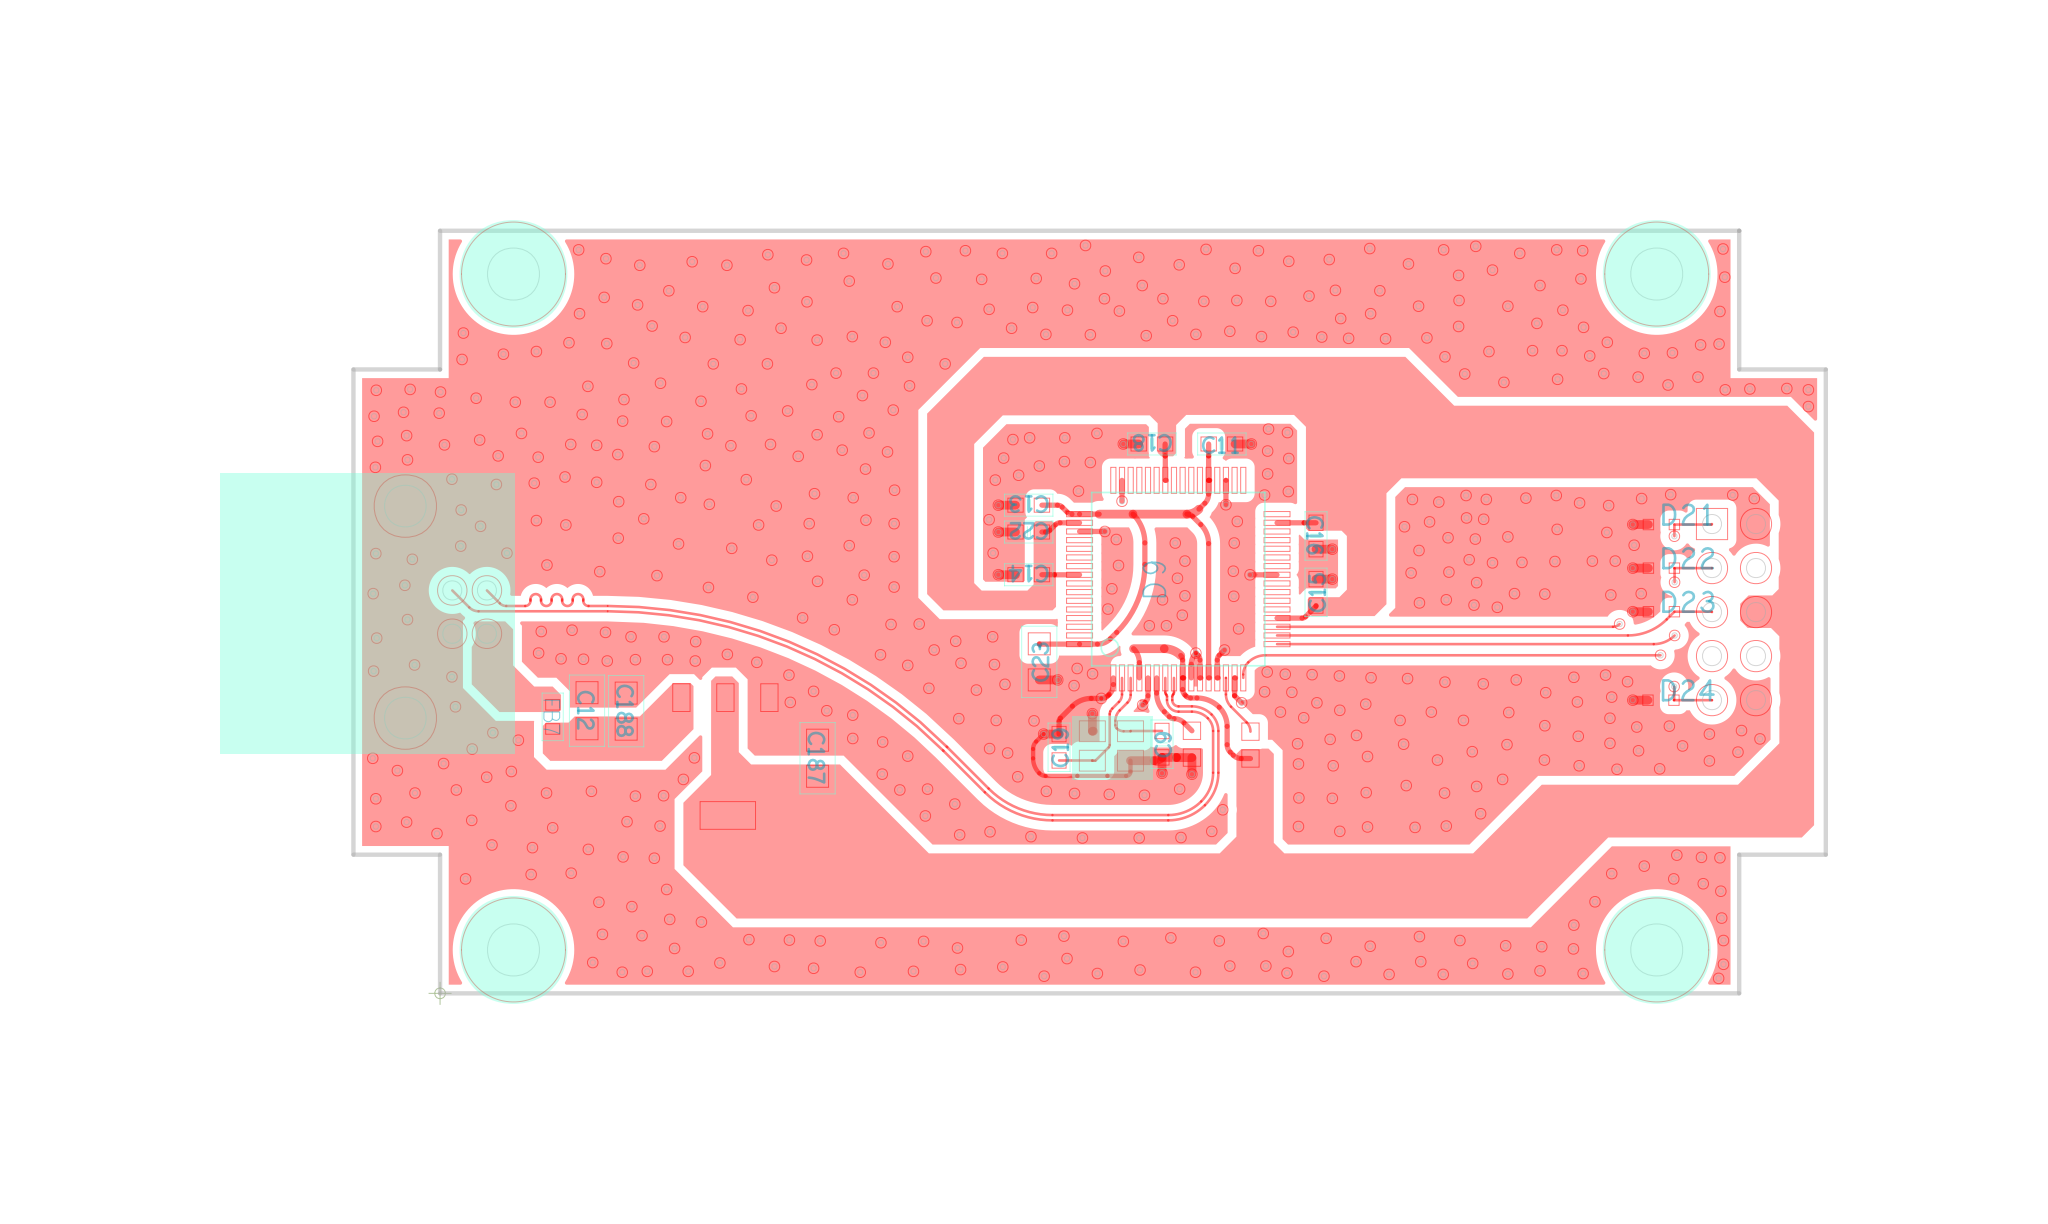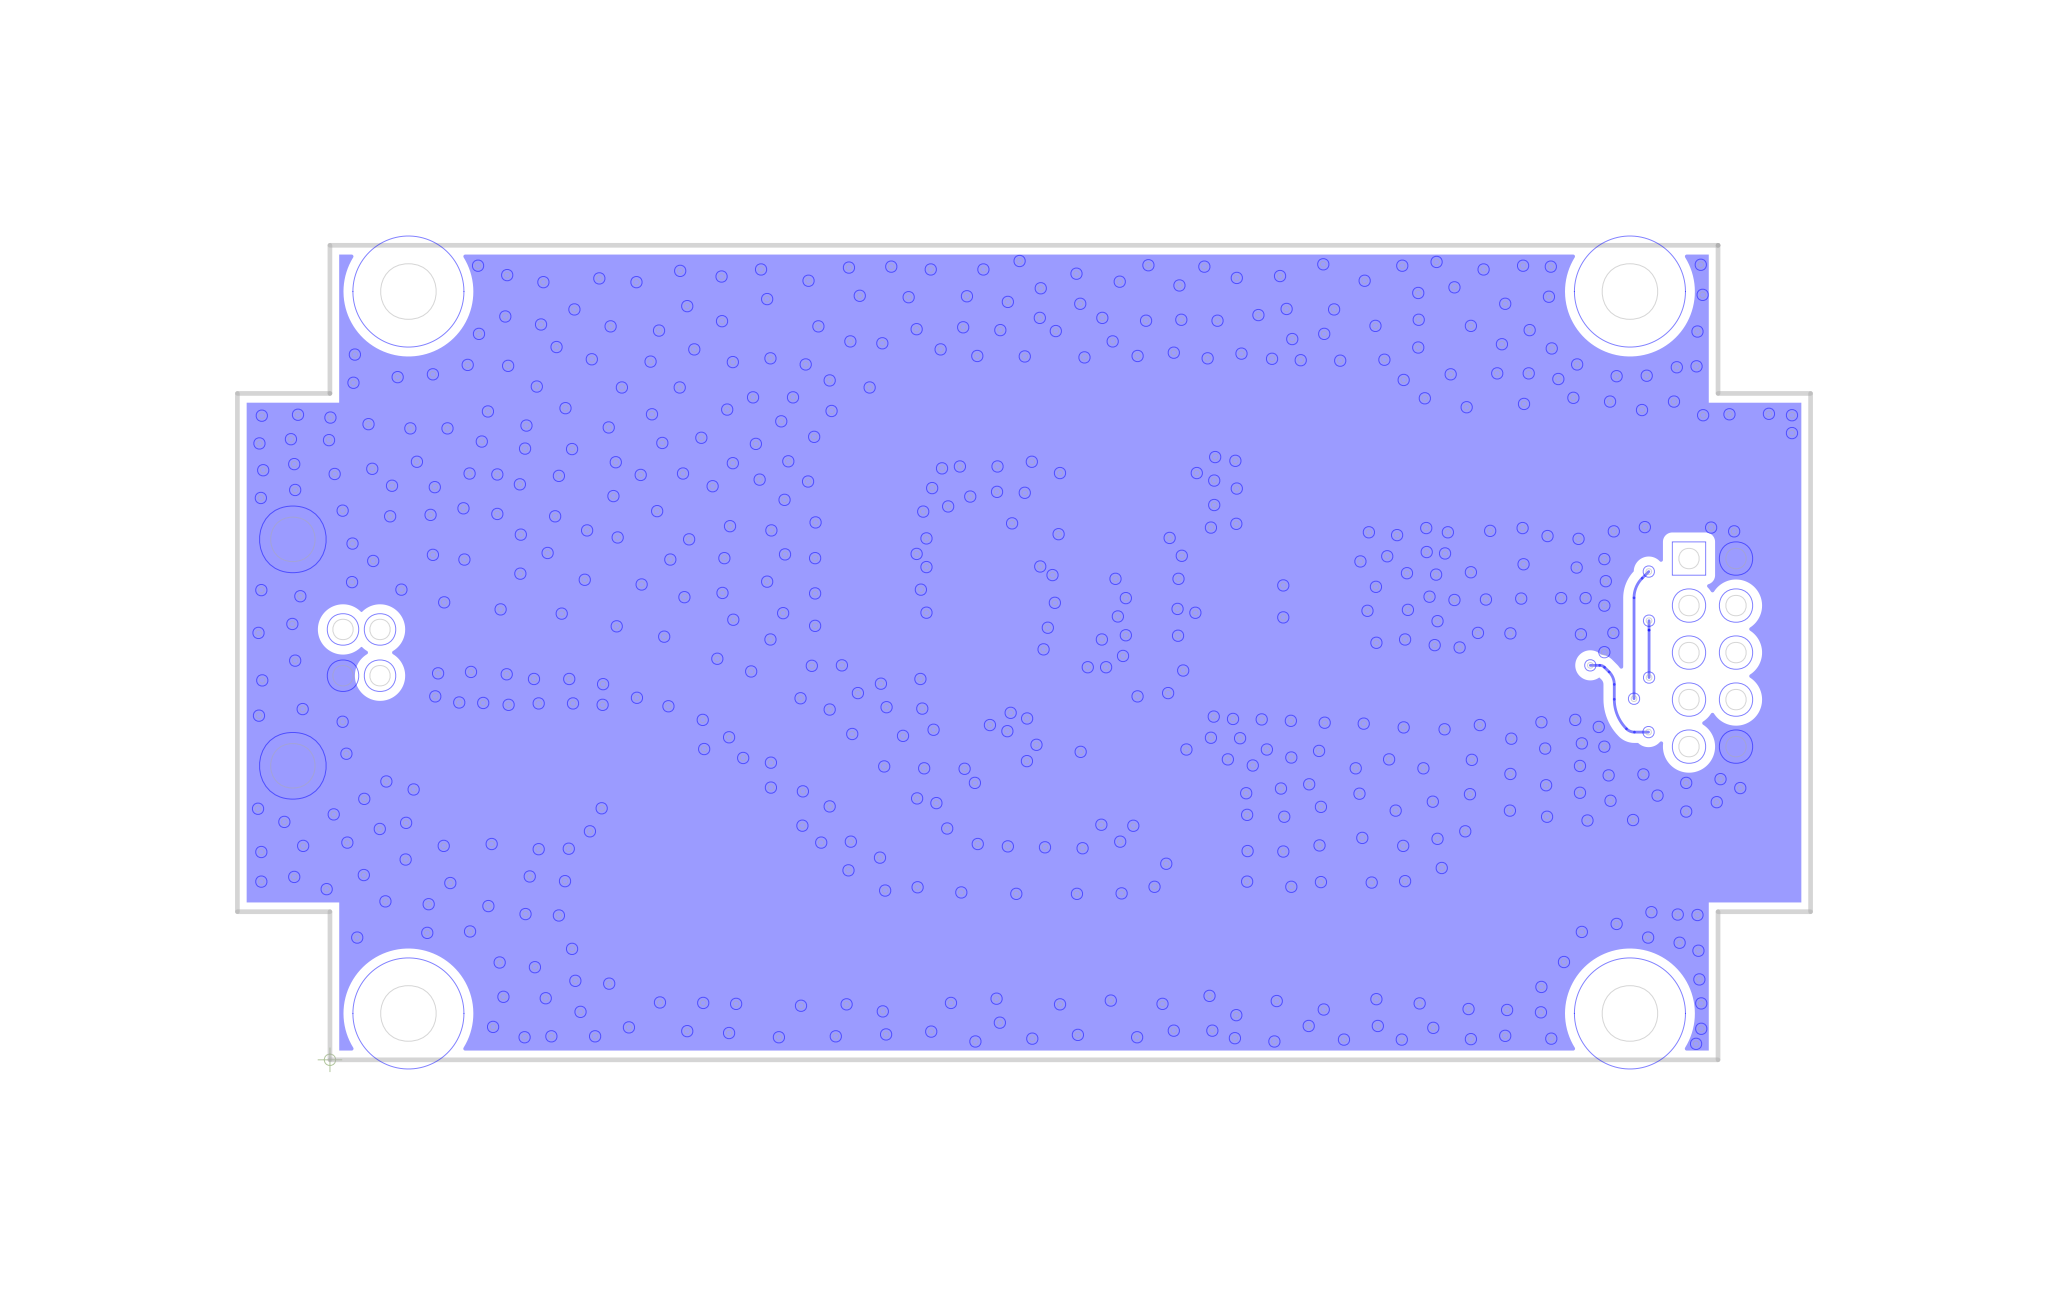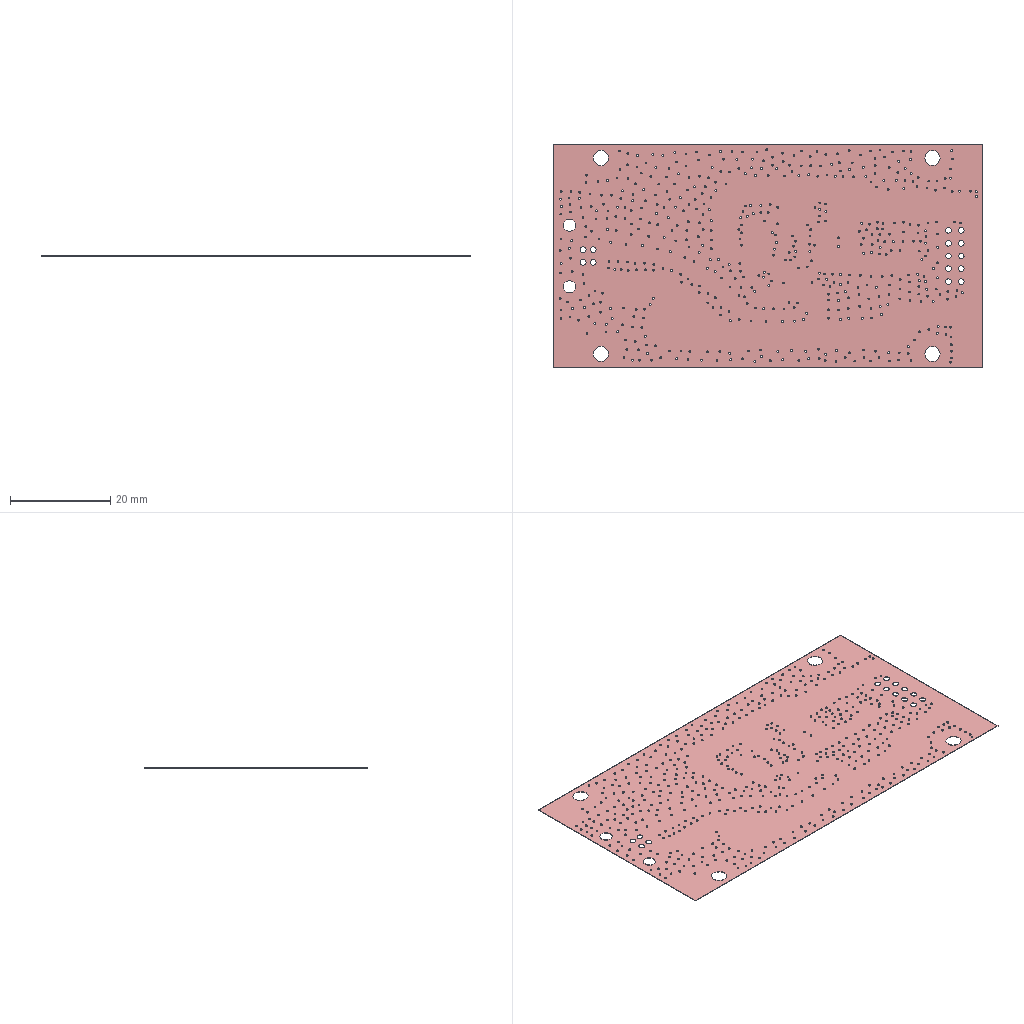Circuit board layout | Cadence Allegro | box 85.3 x 44.3 x 0.1 mm
Layer stack:
# Cadence Allegro layer stack of  (unit mm; from the constraint file cross-section; dielectric type: 0 not recorded (Allegro does not mark core vs prepreg), 3 surface material)
index,name,kind,layer,copper_thickness_mm,dielectric_type,dielectric_thickness_mm,dielectric_material,dielectric_constant
0,Top Surface,other,,,,,,
1,TOP,copper,TOP,0.035,,,,
2,Dielectric1,dielectric,,,0,0.1,FR-4,4.5
3,BOTTOM,copper,BOTTOM,0.035,,,,
4,Bottom Surface,other,,,,,,
# drill layer pairs: low layer,high layer
drill_pair,TOP,BOTTOM
Part placement:
REFDES,COMP_VALUE,SYM_NAME,SYM_X,SYM_Y,SYM_ROTATE,SYM_MIRROR
C9,22pF,SMC0603,1640.902,566.000,90.000,NO
C11,10nF,SMC0603,1776.902,1248.000,0.000,NO
C12,10uF,C0805,334.000,642.098,270.000,NO
C13,100nF,SMC0603,1337.902,1109.000,180.000,NO
C14,100nF,SMC0603,1337.902,951.000,180.000,NO
C15,100nF,SMC0603,1990.902,911.000,90.000,NO
C16,100nF,SMC0603,1990.902,1039.000,270.000,NO
C18,100nF,SMC0603,1617.902,1248.000,180.000,NO
C19,22pF,SMC0603,1406.902,559.000,90.000,NO
C22,100nF,SMC0603,1337.902,1048.000,180.000,NO
C23,10uF,C0805,1361.902,753.000,90.000,NO
C187,10uF,C0805,858.000,534.098,270.000,NO
C188,10uF,C0805,423.000,641.098,270.000,NO
D9,FT2232HL,LQFP64_D12_E12_P0R5,1677.902,941.000,90.000,NO
D20,AMS1117-3.3,SOT-223,654.000,404.098,180.000,NO
D21,BSD5C031V,SOD-523_L1_2-W0_8-LS1_6-BI,2775.902,1065.000,0.000,NO
D22,BSD5C031V,SOD-523_L1_2-W0_8-LS1_6-BI,2775.902,966.000,0.000,NO
D23,BSD5C031V,SOD-523_L1_2-W0_8-LS1_6-BI,2775.902,867.000,0.000,NO
D24,BSD5C031V,SOD-523_L1_2-W0_8-LS1_6-BI,2774.902,666.000,0.000,NO
FB7,MPZ1608S601A NC,FB0603,256.000,628.098,270.000,NO
G1,X322525MSB4SI_C13740,3225,1525.902,562.000,0.000,NO
J1,2.54mm_2x5,IDC-TH_10P-P2_54-H-R2-C5-S2_54,2940.945,866.142,90.000,NO
R185,12K,R0603,1708.902,566.000,90.000,NO
R197,10K,R0603,1841.902,564.000,90.000,NO
X15,usb2.0_B_C46392,USB-B_TH_BF90,13.780,866.142,270.000,NO
Pad and via stacks:
# Allegro (Cadence) via spans and padstacks; design units: ("mils" 3 1000)
# via spans: padstack,start_layer,end_layer,net_example,count
VIA12_24,ETCH/TOP,ETCH/BOTTOM,GND,568
# Allegro padstack definitions: name,start_layer,end_layer,drill,plating,holeType,type
SMD_OV36X30,"ETCH/TOP","ETCH/TOP",0.0,"PLATED","none","smd"
SMD_SQ50,"ETCH/TOP","ETCH/TOP",0.0,"PLATED","none","smd"
SMD10X16,"ETCH/TOP","ETCH/TOP",0.0,"PLATED","none","smd"
SMD32X16,"ETCH/TOP","ETCH/TOP",0.0,"PLATED","none","smd"
SMD0_3X1_5,"ETCH/TOP","ETCH/TOP",0.0,"PLATED","none","smd"
R150_30,"ETCH/TOP","ETCH/TOP",0.0,"PLATED","none","smd"
RECT24X32,"ETCH/TOP","ETCH/TOP",0.0,"PLATED","none","smd"
RECT71X47,"ETCH/TOP","ETCH/TOP",0.0,"PLATED","none","smd"
SMD66X71,"ETCH/TOP","ETCH/TOP",0.0,"PLATED","none","smd"
SMD_SQ32,"ETCH/TOP","ETCH/TOP",0.0,"PLATED","none","smd"
SMD39SQU,"ETCH/TOP","ETCH/TOP",0.0,"NON_PLATED","none","smd"
RECT83X55,"ETCH/TOP","ETCH/TOP",0.0,"PLATED","none","smd"
RE98_42X78_74,"ETCH/TOP","ETCH/TOP",0.0,"NON_PLATED","none","smd"
RE118_11X19_68,"ETCH/TOP","ETCH/TOP",0.0,"NON_PLATED","none","smd"
RECT35X32,"ETCH/TOP","ETCH/TOP",0.0,"PLATED","none","smd"
R150X121,"ETCH/TOP","ETCH/TOP",0.0,"PLATED","none","smd"
SMD_S236P0S40,"ETCH/TOP","ETCH/TOP",0.0,"PLATED","none","smd"
PAD1_8CIR1,"ETCH/TOP","ETCH/BOTTOM",39.402,"PLATED","circle_drill","through"
C054_039,"ETCH/TOP","ETCH/BOTTOM",39.0,"PLATED","circle_drill","through"
S054_039,"ETCH/TOP","ETCH/BOTTOM",39.0,"PLATED","circle_drill","through"
S058_043,"ETCH/TOP","ETCH/BOTTOM",43.0,"PLATED","circle_drill","through"
C058_043,"ETCH/TOP","ETCH/BOTTOM",43.0,"PLATED","circle_drill","through"
VIA,"ETCH/TOP","ETCH/BOTTOM",13.0,"PLATED","circle_drill","through"
TH3P0,"ETCH/TOP","ETCH/BOTTOM",118.11,"PLATED","circle_drill","through"
PLACE-LED3UNIT,"ETCH/TOP","ETCH/BOTTOM",137.799,"PLATED","circle_drill","through"
TH138_CIR118,"ETCH/TOP","ETCH/BOTTOM",137.799,"PLATED","circle_drill","through"
HOLE3P0,"ETCH/TOP","ETCH/BOTTOM",118.11,"PLATED","circle_drill","through"
VIA_10_18,"ETCH/TOP","ETCH/BOTTOM",10.0,"PLATED","circle_drill","through"
PAD60CIR40D_1,"ETCH/TOP","ETCH/BOTTOM",40.0,"PLATED","circle_drill","through"
PAD60SQ40D_1,"ETCH/TOP","ETCH/BOTTOM",40.0,"PLATED","circle_drill","through"
PTH_C669SLOT433X433S40,"ETCH/TOP","ETCH/BOTTOM",43.311,"PLATED","oval slot","through"
PTH_C1221SLOT827X827S40,"ETCH/TOP","ETCH/BOTTOM",82.681,"PLATED","oval slot","through"
HOLE2-3_5,"ETCH/TOP","ETCH/BOTTOM",82.681,"PLATED","circle_drill","through"
PAD158CIR107D,"ETCH/TOP","ETCH/BOTTOM",106.299,"PLATED","circle_drill","through"
VIA12_24,"ETCH/TOP","ETCH/BOTTOM",12.0,"PLATED","circle_drill","through"
PTH_C1417SLOT945X945S40,"ETCH/TOP","ETCH/BOTTOM",94.488,"PLATED","oval slot","through"
PTH_C709SLOT433X433S40,"ETCH/TOP","ETCH/BOTTOM",43.311,"PLATED","oval slot","through"
PTH_S709SLOT433X433S40,"ETCH/TOP","ETCH/BOTTOM",43.311,"PLATED","oval slot","through"
D3,"ETCH/TOP","ETCH/BOTTOM",118.11,"NON_PLATED","circle_drill","through"
C177_17D137_80,"ETCH/TOP","ETCH/BOTTOM",157.48,"PLATED","circle_drill","through"
HOLE5P5D3P2,"ETCH/TOP","ETCH/BOTTOM",125.98,"PLATED","circle_drill","through"
Y300_600,"ETCH/TOP","ETCH/BOTTOM",118.11,"PLATED","circle_drill","through"
Design rules, without the lines most boards share, first 13 of 24 lines:
# Cadence Allegro design rules of  (from the Constraint Manager export constraints.dcfx, design unit mil; typed fields in mm)
# columns: name | kind | enabled | priority | scope1 | scope2 | descriptor | typed fields (field=value)
# Allegro precedence (priority 1 wins): 1 Region class-to-class, 2 Region class, 3 Region, 4 class-to-class, 5 DiffPair/Bus/NetGroup override, 6 NetClass, 7 constraint set (CSet) default
# per-layer values are written LAYER=value in the descriptor and LAYER:mm in the typed field; a maximum of 0 means no limit set
# --- net classes (and buses / net groups) ---
# (no net classes defined: every net uses the default constraint sets)
# --- track widths, neck and differential-pair gap (physical constraint sets) ---
DEFAULT | PhysicalCSet | enabled | 7 | Design default | All | Physical Constraint (Min Line Width=6mil) (Max Line Width=0mil) (Min Neck Width=6mil) (Max Neck Length=0mil) (DiffPair Primary Gap=6mil) (DiffPair Neck Gap=0mil) (DiffPair Min Space=0mil) (DiffPair Coupled +Tol=0mil) (DiffPair Coupled -Tol=0mil) (Min BB Via Stagger=5mil) (Max BB Via Stagger=0mil) (T-junctions=ANYWHERE) (Pad-pad direct connect=ALL_ALLOWED) (Allowed vias=VIA12_24) | min_line_width=0.1524 min_neck_width=0.1524 ts_allowed=ANYWHERE min_bvia_stagger=0.127 max_bvia_stagger=0 diffp_primary_gap=0.1524 diffp_neck_gap=0 diffp_coupled_plus=0 diffp_coupled_minus=0 diffp_min_space=0 max_line_width=0 maximum_neck_length=0 allow_on_etch_subclass=TRUE pad_pad_direct_connect=ALL_ALLOWED vias=VIA12_24
# --- clearances: line / pad / via / shape / hole (spacing constraint sets) ---
DEFAULT | SpacingCSet | enabled | 7 | Design default | All | Clearance Constraint (Line-Line=6mil) (Line-SMD Pad=6mil) (Line-Thru Pin=6mil) (Line-Via=6mil) (Line-Shape=20mil) (SMD Pad-SMD Pad=6mil) (Thru Pin-Thru Pin=6mil) (Thru Pin-SMD Pad=6mil) (SMD Pad-Via=6mil) (Thru Pin-Via=6mil) (Via-Via=6mil) (Shape-SMD Pad=20mil) (Shape-Thru Pin=20mil) (Shape-Via=20mil) (Shape-Shape=20mil) (Hole-Hole=8mil) (Hole-Line=6mil) (Hole-Shape=8mil) (BB Via-BB Via=6mil) (uVia-uVia=5mil) | line_to_line_spacing=0.1524 line_to_smdpin_spacing=0.1524 smdpin_to_smdpin_spacing=0.1524 line_to_testpin_spacing=0.1524 testpin_to_thrupin_spacing=0.1524 testpin_to_testpin_spacing=0.1524 line_to_thruvia_spacing=0.1524 smdpin_to_thruvia_spacing=0.1524 testpin_to_thruvia_spacing=0.1524 thruvia_to_thruvia_spacing=0.1524 bbv_to_line_spacing=0.1524 bbv_to_thrupin_spacing=0.1524 bbv_to_smdpin_spacing=0.1524 bbv_to_testpin_spacing=0.1524 bbv_to_bbv_spacing=0.1524 line_to_testvia_spacing=0.1524 smdpin_to_testvia_spacing=0.1524 testpin_to_testvia_spacing=0.1524 testvia_to_thruvia_spacing=0.1524 bbv_to_testvia_spacing=0.1524 testvia_to_testvia_spacing=0.1524 mvia_to_line_spacing=0.1524 mvia_to_thrupin_spacing=0.127 mvia_to_smdpin_spacing=0.127 mvia_to_testpin_spacing=0.127 mvia_to_thruvia_spacing=0.127 mvia_to_bbv_spacing=0.127 mvia_to_mvia_spacing=0.127 line_to_shape_spacing=0.508 shape_to_smdpin_spacing=0.508 shape_to_testpin_spacing=0.508 shape_to_thruvia_spacing=0.508 bbv_to_shape_spacing=0.508 shape_to_testvia_spacing=0.508 mvia_to_shape_spacing=0.127 shape_to_shape_spacing=0.508 bondpad_to_line_spacing=0.1524 thrupin_to_bondpad_spacing=0.1524 smdpin_to_bondpad_spacing=0.1524 bondpad_to_testpin_spacing=0.1524 bondpad_to_thruvia_spacing=0.1524 bondpad_to_bbv_spacing=0.1524 bondpad_to_testvia_spacing=0.1524 bondpad_to_mvia_spacing=0.127 bondpad_to_bondpad_spacing=0.1524 thrupin_to_thrupin_spacing=0.1524 thrupin_to_smdpin_spacing=0.1524 thrupin_to_thruvia_spacing=0.1524 line_to_thrupin_spacing=0.1524 thrupin_to_shape_spacing=0.508 bbv_to_thruvia_spacing=0.1524 smdpin_to_testpin_spacing=0.1524 testvia_to_thrupin_spacing=0.1524 bondpad_to_shape_spacing=0.508 hole_to_pin_spacing=0.2032 hole_to_via_spacing=0.2032 hole_to_line_spacing=0.1524 hole_to_shape_spacing=0.2032 hole_to_hole_spacing=0.2032 mvia_to_testvia_spacing=0.127 bondpad_to_bondpad_diffp_spc=0.127 min_bvia_gap=0.127
DEFAULT | SameNetSpacingCSet | enabled | 7 | Design default | All | Same-Net Clearance (Line-Line=5mil) (Line-SMD Pad=5mil) (Line-Thru Pin=5mil) (Line-Via=5mil) (Line-Shape=5mil) (SMD Pad-SMD Pad=5mil) (Thru Pin-Thru Pin=5mil) (Thru Pin-SMD Pad=5mil) (SMD Pad-Via=5mil) (Thru Pin-Via=5mil) (Via-Via=5mil) (Shape-SMD Pad=5mil) (Shape-Thru Pin=5mil) (Shape-Via=5mil) (Shape-Shape=5mil) (Hole-Hole=8mil) (Hole-Line=8mil) (Hole-Shape=8mil) (BB Via-BB Via=5mil) (uVia-uVia=5mil) | sn_thrupin_to_thrupin_spacing=0.127 sn_thrupin_to_smdpin_spacing=0.127 sn_thrupin_to_thruvia_spacing=0.127 sn_line_to_thrupin_spacing=0.127 sn_thrupin_to_shape_spacing=0.127 sn_smdpin_to_smdpin_spacing=0.127 sn_smdpin_to_thruvia_spacing=0.127 sn_line_to_smdpin_spacing=0.127 sn_shape_to_smdpin_spacing=0.127 sn_thruvia_to_thruvia_spacing=0.127 sn_line_to_thruvia_spacing=0.127 sn_shape_to_thruvia_spacing=0.127 sn_line_to_line_spacing=0.127 sn_line_to_shape_spacing=0.127 sn_shape_to_shape_spacing=0.127 sn_bbv_to_bbv_spacing=0.127 sn_bbv_to_thrupin_spacing=0.127 sn_bbv_to_smdpin_spacing=0.127 sn_bbv_to_thruvia_spacing=0.127 sn_bbv_to_line_spacing=0.127 sn_bbv_to_shape_spacing=0.127 sn_bbv_to_testpin_spacing=0.127 sn_bbv_to_testvia_spacing=0.127 sn_testpin_to_testpin_spacing=0.127 sn_testpin_to_thrupin_spacing=0.127 sn_smdpin_to_testpin_spacing=0.127 sn_testpin_to_thruvia_spacing=0.127 sn_testpin_to_testvia_spacing=0.127 sn_line_to_testpin_spacing=0.127 sn_shape_to_testpin_spacing=0.127 sn_testvia_to_testvia_spacing=0.127 sn_testvia_to_thrupin_spacing=0.127 sn_smdpin_to_testvia_spacing=0.127 sn_testvia_to_thruvia_spacing=0.127 sn_line_to_testvia_spacing=0.127 sn_shape_to_testvia_spacing=0.127 sn_bondpad_to_bondpad_spacing=0.127 sn_thrupin_to_bondpad_spacing=0.127 sn_smdpin_to_bondpad_spacing=0.127 sn_bondpad_to_thruvia_spacing=0.127 sn_bondpad_to_line_spacing=0.127 sn_bondpad_to_shape_spacing=0.127 sn_bondpad_to_bbv_spacing=0.127 sn_bondpad_to_testpin_spacing=0.127 sn_bondpad_to_testvia_spacing=0.127 same_net=TRUE sn_hole_to_pin_spacing=0.2032 sn_hole_to_via_spacing=0.2032 sn_hole_to_line_spacing=0.2032 sn_hole_to_shape_spacing=0.2032 sn_hole_to_hole_spacing=0.2032 sn_mvia_to_mvia_spacing=0.127 sn_mvia_to_thrupin_spacing=0.127 sn_mvia_to_smdpin_spacing=0.127 sn_mvia_to_thruvia_spacing=0.127 sn_mvia_to_bbv_spacing=0.127 sn_mvia_to_line_spacing=0.127 sn_mvia_to_shape_spacing=0.127 sn_mvia_to_testpin_spacing=0.127 sn_mvia_to_testvia_spacing=0.127 sn_bondpad_to_mvia_spacing=0.127
# --- differential pairs (1) ---
USB_D | DiffPair | enabled | 5 | USB_D+ | USB_D- | Differential Pair (Primary Gap=6mil) (Min Line Width=6mil) (Physical CSet=DEFAULT) overrides: (DIFFP_PHASE_TOL=2.5 mil) (MIN_LINE_WIDTH=6mil) | gap=0.1524 width=0.1524 electricalcset=ECS1 diffp_phase_tol=2.5mil min_line_width=0.1524